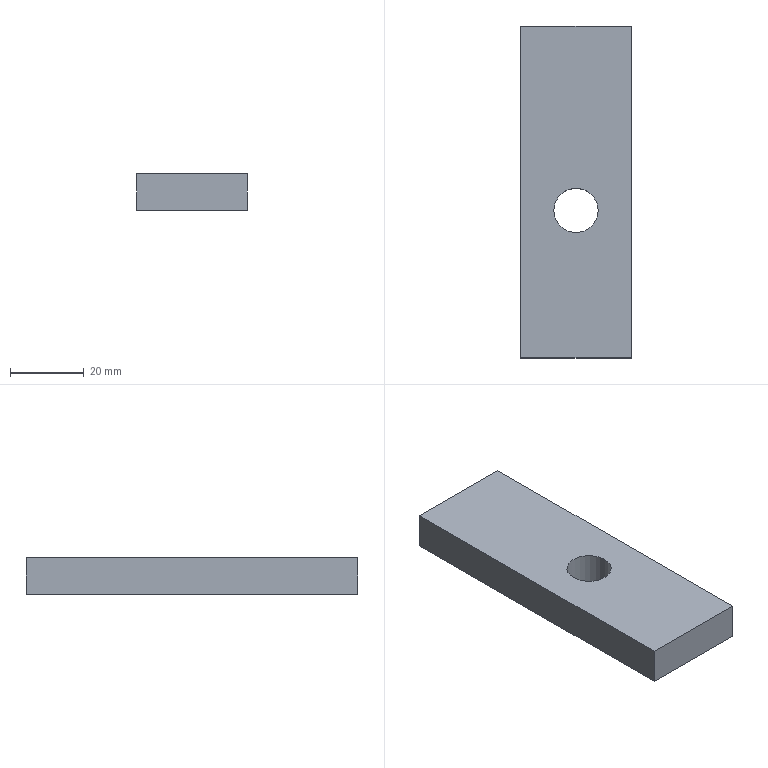Part | NX | features solid 2 | 1 solid | 7 faces | box 30 x 90 x 10 mm | volume 25869 mm3 | plane 6 | cylinder 1 | commonest cylinder face diameters 12 x1
STEP:
#1=CARTESIAN_POINT('',(-510.,-55.,-65.));
#2=VERTEX_POINT('',#1);
#3=CARTESIAN_POINT('',(-510.,-55.,-55.));
#4=VERTEX_POINT('',#3);
#5=CARTESIAN_POINT('',(-510.,-55.,0.));
#6=DIRECTION('',(0.,0.,-1.));
#7=VECTOR('',#6,1000.);
#8=LINE('',#5,#7);
#9=EDGE_CURVE('',#2,#4,#8,.F.);
#10=ORIENTED_EDGE('',*,*,#9,.F.);
#11=CARTESIAN_POINT('',(-540.,-55.,-65.));
#12=VERTEX_POINT('',#11);
#13=CARTESIAN_POINT('',(-610.,-55.,-65.));
#14=DIRECTION('',(-1.,0.,0.));
#15=VECTOR('',#14,1000.);
#16=LINE('',#13,#15);
#17=EDGE_CURVE('',#12,#2,#16,.F.);
#18=ORIENTED_EDGE('',*,*,#17,.F.);
#19=CARTESIAN_POINT('',(-540.,-55.,-55.));
#20=VERTEX_POINT('',#19);
#21=CARTESIAN_POINT('',(-540.,-55.,0.));
#22=DIRECTION('',(0.,0.,1.));
#23=VECTOR('',#22,1000.);
#24=LINE('',#21,#23);
#25=EDGE_CURVE('',#20,#12,#24,.F.);
#26=ORIENTED_EDGE('',*,*,#25,.F.);
#27=CARTESIAN_POINT('',(-610.,-55.,-55.));
#28=DIRECTION('',(-1.,0.,0.));
#29=VECTOR('',#28,1000.);
#30=LINE('',#27,#29);
#31=EDGE_CURVE('',#4,#20,#30,.T.);
#32=ORIENTED_EDGE('',*,*,#31,.F.);
#33=EDGE_LOOP('',(#10,#18,#26,#32));
#34=FACE_BOUND('',#33,.T.);
#35=CARTESIAN_POINT('',(-525.,-55.,0.));
#36=DIRECTION('',(0.,-1.,0.));
#37=DIRECTION('',(0.,0.,-1.));
#38=AXIS2_PLACEMENT_3D('',#35,#36,#37);
#39=PLANE('',#38);
#40=ADVANCED_FACE('',(#34),#39,.F.);
#41=CARTESIAN_POINT('',(-531.,-105.,-65.));
#42=VERTEX_POINT('',#41);
#43=CARTESIAN_POINT('',(-525.,-105.,-65.));
#44=DIRECTION('',(0.,0.,-1.));
#45=DIRECTION('',(-1.,0.,0.));
#46=AXIS2_PLACEMENT_3D('',#43,#44,#45);
#47=CIRCLE('',#46,6.);
#48=EDGE_CURVE('',#42,#42,#47,.F.);
#49=ORIENTED_EDGE('',*,*,#48,.F.);
#50=EDGE_LOOP('',(#49));
#51=FACE_BOUND('',#50,.T.);
#52=CARTESIAN_POINT('',(-531.,-105.,-55.));
#53=VERTEX_POINT('',#52);
#54=CARTESIAN_POINT('',(-525.,-105.,-55.));
#55=DIRECTION('',(0.,0.,-1.));
#56=DIRECTION('',(-1.,0.,0.));
#57=AXIS2_PLACEMENT_3D('',#54,#55,#56);
#58=CIRCLE('',#57,6.);
#59=EDGE_CURVE('',#53,#53,#58,.F.);
#60=ORIENTED_EDGE('',*,*,#59,.T.);
#61=EDGE_LOOP('',(#60));
#62=FACE_BOUND('',#61,.T.);
#63=CARTESIAN_POINT('',(-525.,-105.,0.));
#64=DIRECTION('',(0.,0.,-1.));
#65=DIRECTION('',(-1.,0.,0.));
#66=AXIS2_PLACEMENT_3D('',#63,#64,#65);
#67=CYLINDRICAL_SURFACE('',#66,6.);
#68=ADVANCED_FACE('',(#51,#62),#67,.F.);
#69=ORIENTED_EDGE('',*,*,#59,.F.);
#70=EDGE_LOOP('',(#69));
#71=FACE_BOUND('',#70,.T.);
#72=CARTESIAN_POINT('',(-510.,-145.,-55.));
#73=VERTEX_POINT('',#72);
#74=CARTESIAN_POINT('',(-510.,-25.,-55.));
#75=DIRECTION('',(0.,1.,0.));
#76=VECTOR('',#75,1000.);
#77=LINE('',#74,#76);
#78=EDGE_CURVE('',#4,#73,#77,.F.);
#79=ORIENTED_EDGE('',*,*,#78,.F.);
#80=ORIENTED_EDGE('',*,*,#31,.T.);
#81=CARTESIAN_POINT('',(-540.,-145.,-55.));
#82=VERTEX_POINT('',#81);
#83=CARTESIAN_POINT('',(-540.,-25.,-55.));
#84=DIRECTION('',(0.,1.,0.));
#85=VECTOR('',#84,1000.);
#86=LINE('',#83,#85);
#87=EDGE_CURVE('',#20,#82,#86,.F.);
#88=ORIENTED_EDGE('',*,*,#87,.T.);
#89=CARTESIAN_POINT('',(-610.,-145.,-55.));
#90=DIRECTION('',(1.,0.,0.));
#91=VECTOR('',#90,1000.);
#92=LINE('',#89,#91);
#93=EDGE_CURVE('',#82,#73,#92,.T.);
#94=ORIENTED_EDGE('',*,*,#93,.T.);
#95=EDGE_LOOP('',(#79,#80,#88,#94));
#96=FACE_BOUND('',#95,.T.);
#97=CARTESIAN_POINT('',(-610.,110.,-55.));
#98=DIRECTION('',(0.,0.,-1.));
#99=DIRECTION('',(0.,1.,0.));
#100=AXIS2_PLACEMENT_3D('',#97,#98,#99);
#101=PLANE('',#100);
#102=ADVANCED_FACE('',(#71,#96),#101,.F.);
#103=CARTESIAN_POINT('',(-540.,-145.,-65.));
#104=VERTEX_POINT('',#103);
#105=CARTESIAN_POINT('',(-540.,-145.,0.));
#106=DIRECTION('',(0.,0.,1.));
#107=VECTOR('',#106,1000.);
#108=LINE('',#105,#107);
#109=EDGE_CURVE('',#82,#104,#108,.F.);
#110=ORIENTED_EDGE('',*,*,#109,.F.);
#111=ORIENTED_EDGE('',*,*,#87,.F.);
#112=ORIENTED_EDGE('',*,*,#25,.T.);
#113=CARTESIAN_POINT('',(-540.,90.,-65.));
#114=DIRECTION('',(0.,1.,0.));
#115=VECTOR('',#114,1000.);
#116=LINE('',#113,#115);
#117=EDGE_CURVE('',#12,#104,#116,.F.);
#118=ORIENTED_EDGE('',*,*,#117,.T.);
#119=EDGE_LOOP('',(#110,#111,#112,#118));
#120=FACE_BOUND('',#119,.T.);
#121=CARTESIAN_POINT('',(-540.,90.,0.));
#122=DIRECTION('',(1.,0.,0.));
#123=DIRECTION('',(0.,0.,-1.));
#124=AXIS2_PLACEMENT_3D('',#121,#122,#123);
#125=PLANE('',#124);
#126=ADVANCED_FACE('',(#120),#125,.F.);
#127=ORIENTED_EDGE('',*,*,#78,.T.);
#128=CARTESIAN_POINT('',(-510.,-145.,-65.));
#129=VERTEX_POINT('',#128);
#130=CARTESIAN_POINT('',(-510.,-145.,0.));
#131=DIRECTION('',(0.,0.,1.));
#132=VECTOR('',#131,1000.);
#133=LINE('',#130,#132);
#134=EDGE_CURVE('',#73,#129,#133,.F.);
#135=ORIENTED_EDGE('',*,*,#134,.T.);
#136=CARTESIAN_POINT('',(-510.,90.,-65.));
#137=DIRECTION('',(0.,1.,0.));
#138=VECTOR('',#137,1000.);
#139=LINE('',#136,#138);
#140=EDGE_CURVE('',#2,#129,#139,.F.);
#141=ORIENTED_EDGE('',*,*,#140,.F.);
#142=ORIENTED_EDGE('',*,*,#9,.T.);
#143=EDGE_LOOP('',(#127,#135,#141,#142));
#144=FACE_BOUND('',#143,.T.);
#145=CARTESIAN_POINT('',(-510.,90.,0.));
#146=DIRECTION('',(1.,0.,0.));
#147=DIRECTION('',(0.,0.,-1.));
#148=AXIS2_PLACEMENT_3D('',#145,#146,#147);
#149=PLANE('',#148);
#150=ADVANCED_FACE('',(#144),#149,.T.);
#151=ORIENTED_EDGE('',*,*,#48,.T.);
#152=EDGE_LOOP('',(#151));
#153=FACE_BOUND('',#152,.T.);
#154=ORIENTED_EDGE('',*,*,#140,.T.);
#155=CARTESIAN_POINT('',(-610.,-145.,-65.));
#156=DIRECTION('',(1.,0.,0.));
#157=VECTOR('',#156,1000.);
#158=LINE('',#155,#157);
#159=EDGE_CURVE('',#129,#104,#158,.F.);
#160=ORIENTED_EDGE('',*,*,#159,.T.);
#161=ORIENTED_EDGE('',*,*,#117,.F.);
#162=ORIENTED_EDGE('',*,*,#17,.T.);
#163=EDGE_LOOP('',(#154,#160,#161,#162));
#164=FACE_BOUND('',#163,.T.);
#165=CARTESIAN_POINT('',(-610.,110.,-65.));
#166=DIRECTION('',(0.,0.,-1.));
#167=DIRECTION('',(0.,1.,0.));
#168=AXIS2_PLACEMENT_3D('',#165,#166,#167);
#169=PLANE('',#168);
#170=ADVANCED_FACE('',(#153,#164),#169,.T.);
#171=ORIENTED_EDGE('',*,*,#93,.F.);
#172=ORIENTED_EDGE('',*,*,#109,.T.);
#173=ORIENTED_EDGE('',*,*,#159,.F.);
#174=ORIENTED_EDGE('',*,*,#134,.F.);
#175=EDGE_LOOP('',(#171,#172,#173,#174));
#176=FACE_BOUND('',#175,.T.);
#177=CARTESIAN_POINT('',(-510.,-145.,0.));
#178=DIRECTION('',(0.,1.,0.));
#179=DIRECTION('',(0.,0.,1.));
#180=AXIS2_PLACEMENT_3D('',#177,#178,#179);
#181=PLANE('',#180);
#182=ADVANCED_FACE('',(#176),#181,.F.);
#183=CLOSED_SHELL('',(#40,#68,#102,#126,#150,#170,#182));
#184=MANIFOLD_SOLID_BREP('',#183);
#185=(LENGTH_UNIT()NAMED_UNIT(*)SI_UNIT(.MILLI.,.METRE.));
#186=UNCERTAINTY_MEASURE_WITH_UNIT(LENGTH_MEASURE(0.00001),#185,'','');
#187=(NAMED_UNIT(*)PLANE_ANGLE_UNIT()SI_UNIT($,.RADIAN.));
#188=(NAMED_UNIT(*)SI_UNIT($,.STERADIAN.)SOLID_ANGLE_UNIT());
#189=(GEOMETRIC_REPRESENTATION_CONTEXT(3)GLOBAL_UNCERTAINTY_ASSIGNED_CONTEXT((#186))GLOBAL_UNIT_ASSIGNED_CONTEXT((#185,#187,#188))REPRESENTATION_CONTEXT('',''));
#190=ADVANCED_BREP_SHAPE_REPRESENTATION('',(#184),#189);